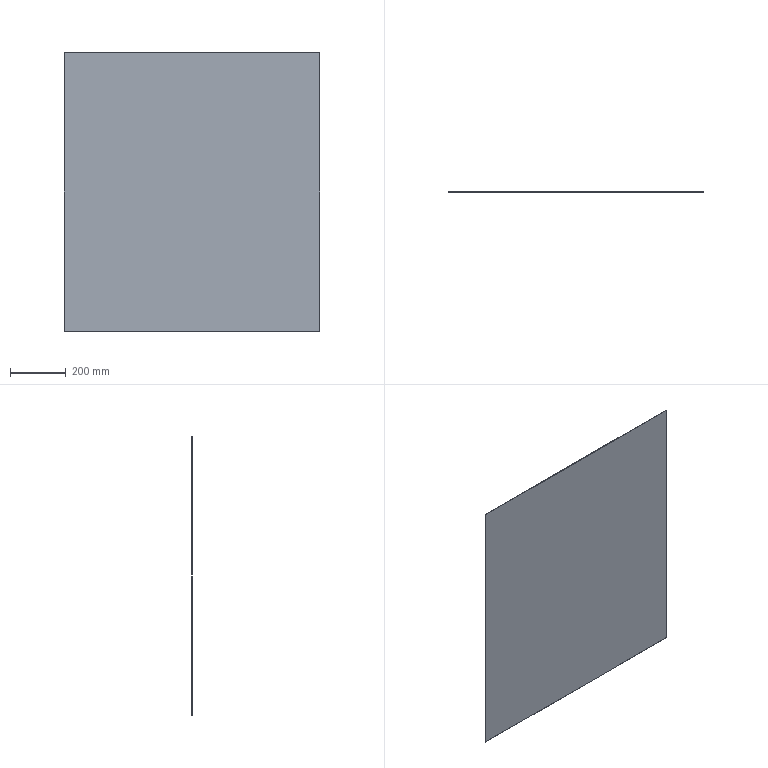Part | STEP file | 0243_Work-A | 1 solid | 6 faces | box 919 x 2.2 x 1000 mm | volume 2021800 mm3 | plane 6
STEP:
#1=CARTESIAN_POINT('',(0.,0.,0.));
#2=DIRECTION('',(0.,0.,1.));
#3=DIRECTION('',(1.,0.,0.));
#4=AXIS2_PLACEMENT_3D('',#1,#2,#3);
#5=CARTESIAN_POINT('',(0.,0.,-500.));
#6=VERTEX_POINT('',#5);
#7=CARTESIAN_POINT('',(0.,0.,500.));
#8=VERTEX_POINT('',#7);
#9=CARTESIAN_POINT('',(0.,0.,500.));
#10=DIRECTION('',(0.,0.,1.));
#11=VECTOR('',#10,1.);
#12=LINE('',#9,#11);
#13=CARTESIAN_POINT('',(0.,2.2,500.));
#14=DIRECTION('',(1.,0.,0.));
#15=DIRECTION('',(0.,0.,-1.));
#16=AXIS2_PLACEMENT_3D('',#13,#14,#15);
#17=PLANE('',#16);
#18=CARTESIAN_POINT('',(0.,-2.2));
#19=DIRECTION('',(-1.,0.));
#20=VECTOR('',#19,1.);
#21=LINE('',#18,#20);
#22=(GEOMETRIC_REPRESENTATION_CONTEXT(2)PARAMETRIC_REPRESENTATION_CONTEXT()REPRESENTATION_CONTEXT('',''));
#23=DEFINITIONAL_REPRESENTATION('',(#21),#22);
#24=PCURVE('',#17,#23);
#25=CARTESIAN_POINT('',(0.,0.,-500.));
#26=DIRECTION('',(0.,-1.,0.));
#27=DIRECTION('',(0.,0.,-1.));
#28=AXIS2_PLACEMENT_3D('',#25,#26,#27);
#29=PLANE('',#28);
#30=CARTESIAN_POINT('',(-1000.,0.));
#31=DIRECTION('',(-1.,0.));
#32=VECTOR('',#31,1.);
#33=LINE('',#30,#32);
#34=(GEOMETRIC_REPRESENTATION_CONTEXT(2)PARAMETRIC_REPRESENTATION_CONTEXT()REPRESENTATION_CONTEXT('',''));
#35=DEFINITIONAL_REPRESENTATION('',(#33),#34);
#36=PCURVE('',#29,#35);
#37=SURFACE_CURVE('',#12,(#24,#36),.PCURVE_S1.);
#38=EDGE_CURVE('',#6,#8,#37,.T.);
#39=ORIENTED_EDGE('',*,*,#38,.T.);
#40=CARTESIAN_POINT('',(0.,2.2,500.));
#41=VERTEX_POINT('',#40);
#42=CARTESIAN_POINT('',(0.,2.2,500.));
#43=DIRECTION('',(0.,-1.,0.));
#44=VECTOR('',#43,1.);
#45=LINE('',#42,#44);
#46=CARTESIAN_POINT('',(0.,0.));
#47=DIRECTION('',(0.,-1.));
#48=VECTOR('',#47,1.);
#49=LINE('',#46,#48);
#50=(GEOMETRIC_REPRESENTATION_CONTEXT(2)PARAMETRIC_REPRESENTATION_CONTEXT()REPRESENTATION_CONTEXT('',''));
#51=DEFINITIONAL_REPRESENTATION('',(#49),#50);
#52=PCURVE('',#17,#51);
#53=CARTESIAN_POINT('',(0.,2.2,500.));
#54=DIRECTION('',(0.,0.,-1.));
#55=DIRECTION('',(-1.,0.,0.));
#56=AXIS2_PLACEMENT_3D('',#53,#54,#55);
#57=PLANE('',#56);
#58=CARTESIAN_POINT('',(0.,0.));
#59=DIRECTION('',(0.,-1.));
#60=VECTOR('',#59,1.);
#61=LINE('',#58,#60);
#62=(GEOMETRIC_REPRESENTATION_CONTEXT(2)PARAMETRIC_REPRESENTATION_CONTEXT()REPRESENTATION_CONTEXT('',''));
#63=DEFINITIONAL_REPRESENTATION('',(#61),#62);
#64=PCURVE('',#57,#63);
#65=SURFACE_CURVE('',#45,(#52,#64),.PCURVE_S1.);
#66=EDGE_CURVE('',#41,#8,#65,.T.);
#67=ORIENTED_EDGE('',*,*,#66,.F.);
#68=CARTESIAN_POINT('',(0.,2.2,-500.));
#69=VERTEX_POINT('',#68);
#70=CARTESIAN_POINT('',(0.,2.2,500.));
#71=DIRECTION('',(0.,0.,1.));
#72=VECTOR('',#71,1.);
#73=LINE('',#70,#72);
#74=CARTESIAN_POINT('',(0.,0.));
#75=DIRECTION('',(-1.,0.));
#76=VECTOR('',#75,1.);
#77=LINE('',#74,#76);
#78=(GEOMETRIC_REPRESENTATION_CONTEXT(2)PARAMETRIC_REPRESENTATION_CONTEXT()REPRESENTATION_CONTEXT('',''));
#79=DEFINITIONAL_REPRESENTATION('',(#77),#78);
#80=PCURVE('',#17,#79);
#81=CARTESIAN_POINT('',(0.,2.2,-500.));
#82=DIRECTION('',(0.,-1.,0.));
#83=DIRECTION('',(0.,0.,-1.));
#84=AXIS2_PLACEMENT_3D('',#81,#82,#83);
#85=PLANE('',#84);
#86=CARTESIAN_POINT('',(-1000.,0.));
#87=DIRECTION('',(-1.,0.));
#88=VECTOR('',#87,1.);
#89=LINE('',#86,#88);
#90=(GEOMETRIC_REPRESENTATION_CONTEXT(2)PARAMETRIC_REPRESENTATION_CONTEXT()REPRESENTATION_CONTEXT('',''));
#91=DEFINITIONAL_REPRESENTATION('',(#89),#90);
#92=PCURVE('',#85,#91);
#93=SURFACE_CURVE('',#73,(#80,#92),.PCURVE_S1.);
#94=EDGE_CURVE('',#69,#41,#93,.T.);
#95=ORIENTED_EDGE('',*,*,#94,.F.);
#96=CARTESIAN_POINT('',(0.,2.2,-500.));
#97=DIRECTION('',(0.,-1.,0.));
#98=VECTOR('',#97,1.);
#99=LINE('',#96,#98);
#100=CARTESIAN_POINT('',(1000.,0.));
#101=DIRECTION('',(0.,-1.));
#102=VECTOR('',#101,1.);
#103=LINE('',#100,#102);
#104=(GEOMETRIC_REPRESENTATION_CONTEXT(2)PARAMETRIC_REPRESENTATION_CONTEXT()REPRESENTATION_CONTEXT('',''));
#105=DEFINITIONAL_REPRESENTATION('',(#103),#104);
#106=PCURVE('',#17,#105);
#107=CARTESIAN_POINT('',(0.,2.2,-500.));
#108=DIRECTION('',(0.,0.,1.));
#109=DIRECTION('',(1.,0.,0.));
#110=AXIS2_PLACEMENT_3D('',#107,#108,#109);
#111=PLANE('',#110);
#112=CARTESIAN_POINT('',(0.,0.));
#113=DIRECTION('',(0.,-1.));
#114=VECTOR('',#113,1.);
#115=LINE('',#112,#114);
#116=(GEOMETRIC_REPRESENTATION_CONTEXT(2)PARAMETRIC_REPRESENTATION_CONTEXT()REPRESENTATION_CONTEXT('',''));
#117=DEFINITIONAL_REPRESENTATION('',(#115),#116);
#118=PCURVE('',#111,#117);
#119=SURFACE_CURVE('',#99,(#106,#118),.PCURVE_S1.);
#120=EDGE_CURVE('',#69,#6,#119,.T.);
#121=ORIENTED_EDGE('',*,*,#120,.T.);
#122=EDGE_LOOP('',(#39,#67,#95,#121));
#123=FACE_BOUND('',#122,.T.);
#124=ADVANCED_FACE('',(#123),#17,.F.);
#125=CARTESIAN_POINT('',(919.,0.,500.));
#126=VERTEX_POINT('',#125);
#127=CARTESIAN_POINT('',(0.,0.,500.));
#128=DIRECTION('',(1.,0.,0.));
#129=VECTOR('',#128,1.);
#130=LINE('',#127,#129);
#131=CARTESIAN_POINT('',(0.,-2.2));
#132=DIRECTION('',(-1.,0.));
#133=VECTOR('',#132,1.);
#134=LINE('',#131,#133);
#135=(GEOMETRIC_REPRESENTATION_CONTEXT(2)PARAMETRIC_REPRESENTATION_CONTEXT()REPRESENTATION_CONTEXT('',''));
#136=DEFINITIONAL_REPRESENTATION('',(#134),#135);
#137=PCURVE('',#57,#136);
#138=CARTESIAN_POINT('',(-1000.,0.));
#139=DIRECTION('',(0.,1.));
#140=VECTOR('',#139,1.);
#141=LINE('',#138,#140);
#142=(GEOMETRIC_REPRESENTATION_CONTEXT(2)PARAMETRIC_REPRESENTATION_CONTEXT()REPRESENTATION_CONTEXT('',''));
#143=DEFINITIONAL_REPRESENTATION('',(#141),#142);
#144=PCURVE('',#29,#143);
#145=SURFACE_CURVE('',#130,(#137,#144),.PCURVE_S1.);
#146=EDGE_CURVE('',#8,#126,#145,.T.);
#147=ORIENTED_EDGE('',*,*,#146,.T.);
#148=CARTESIAN_POINT('',(919.,2.2,500.));
#149=VERTEX_POINT('',#148);
#150=CARTESIAN_POINT('',(919.,2.2,500.));
#151=DIRECTION('',(0.,-1.,0.));
#152=VECTOR('',#151,1.);
#153=LINE('',#150,#152);
#154=CARTESIAN_POINT('',(-919.,0.));
#155=DIRECTION('',(0.,-1.));
#156=VECTOR('',#155,1.);
#157=LINE('',#154,#156);
#158=(GEOMETRIC_REPRESENTATION_CONTEXT(2)PARAMETRIC_REPRESENTATION_CONTEXT()REPRESENTATION_CONTEXT('',''));
#159=DEFINITIONAL_REPRESENTATION('',(#157),#158);
#160=PCURVE('',#57,#159);
#161=CARTESIAN_POINT('',(919.,2.2,500.));
#162=DIRECTION('',(-1.,0.,0.));
#163=DIRECTION('',(0.,0.,1.));
#164=AXIS2_PLACEMENT_3D('',#161,#162,#163);
#165=PLANE('',#164);
#166=CARTESIAN_POINT('',(0.,0.));
#167=DIRECTION('',(0.,-1.));
#168=VECTOR('',#167,1.);
#169=LINE('',#166,#168);
#170=(GEOMETRIC_REPRESENTATION_CONTEXT(2)PARAMETRIC_REPRESENTATION_CONTEXT()REPRESENTATION_CONTEXT('',''));
#171=DEFINITIONAL_REPRESENTATION('',(#169),#170);
#172=PCURVE('',#165,#171);
#173=SURFACE_CURVE('',#153,(#160,#172),.PCURVE_S1.);
#174=EDGE_CURVE('',#149,#126,#173,.T.);
#175=ORIENTED_EDGE('',*,*,#174,.F.);
#176=CARTESIAN_POINT('',(0.,2.2,500.));
#177=DIRECTION('',(1.,0.,0.));
#178=VECTOR('',#177,1.);
#179=LINE('',#176,#178);
#180=CARTESIAN_POINT('',(0.,0.));
#181=DIRECTION('',(-1.,0.));
#182=VECTOR('',#181,1.);
#183=LINE('',#180,#182);
#184=(GEOMETRIC_REPRESENTATION_CONTEXT(2)PARAMETRIC_REPRESENTATION_CONTEXT()REPRESENTATION_CONTEXT('',''));
#185=DEFINITIONAL_REPRESENTATION('',(#183),#184);
#186=PCURVE('',#57,#185);
#187=CARTESIAN_POINT('',(-1000.,0.));
#188=DIRECTION('',(0.,1.));
#189=VECTOR('',#188,1.);
#190=LINE('',#187,#189);
#191=(GEOMETRIC_REPRESENTATION_CONTEXT(2)PARAMETRIC_REPRESENTATION_CONTEXT()REPRESENTATION_CONTEXT('',''));
#192=DEFINITIONAL_REPRESENTATION('',(#190),#191);
#193=PCURVE('',#85,#192);
#194=SURFACE_CURVE('',#179,(#186,#193),.PCURVE_S1.);
#195=EDGE_CURVE('',#41,#149,#194,.T.);
#196=ORIENTED_EDGE('',*,*,#195,.F.);
#197=ORIENTED_EDGE('',*,*,#66,.T.);
#198=EDGE_LOOP('',(#147,#175,#196,#197));
#199=FACE_BOUND('',#198,.T.);
#200=ADVANCED_FACE('',(#199),#57,.F.);
#201=CARTESIAN_POINT('',(919.,0.,-500.));
#202=VERTEX_POINT('',#201);
#203=CARTESIAN_POINT('',(919.,0.,500.));
#204=DIRECTION('',(0.,0.,-1.));
#205=VECTOR('',#204,1.);
#206=LINE('',#203,#205);
#207=CARTESIAN_POINT('',(0.,-2.2));
#208=DIRECTION('',(-1.,0.));
#209=VECTOR('',#208,1.);
#210=LINE('',#207,#209);
#211=(GEOMETRIC_REPRESENTATION_CONTEXT(2)PARAMETRIC_REPRESENTATION_CONTEXT()REPRESENTATION_CONTEXT('',''));
#212=DEFINITIONAL_REPRESENTATION('',(#210),#211);
#213=PCURVE('',#165,#212);
#214=CARTESIAN_POINT('',(-1000.,919.));
#215=DIRECTION('',(1.,0.));
#216=VECTOR('',#215,1.);
#217=LINE('',#214,#216);
#218=(GEOMETRIC_REPRESENTATION_CONTEXT(2)PARAMETRIC_REPRESENTATION_CONTEXT()REPRESENTATION_CONTEXT('',''));
#219=DEFINITIONAL_REPRESENTATION('',(#217),#218);
#220=PCURVE('',#29,#219);
#221=SURFACE_CURVE('',#206,(#213,#220),.PCURVE_S1.);
#222=EDGE_CURVE('',#126,#202,#221,.T.);
#223=ORIENTED_EDGE('',*,*,#222,.T.);
#224=CARTESIAN_POINT('',(919.,2.2,-500.));
#225=VERTEX_POINT('',#224);
#226=CARTESIAN_POINT('',(919.,2.2,-500.));
#227=DIRECTION('',(0.,-1.,0.));
#228=VECTOR('',#227,1.);
#229=LINE('',#226,#228);
#230=CARTESIAN_POINT('',(-1000.,0.));
#231=DIRECTION('',(0.,-1.));
#232=VECTOR('',#231,1.);
#233=LINE('',#230,#232);
#234=(GEOMETRIC_REPRESENTATION_CONTEXT(2)PARAMETRIC_REPRESENTATION_CONTEXT()REPRESENTATION_CONTEXT('',''));
#235=DEFINITIONAL_REPRESENTATION('',(#233),#234);
#236=PCURVE('',#165,#235);
#237=CARTESIAN_POINT('',(919.,0.));
#238=DIRECTION('',(0.,-1.));
#239=VECTOR('',#238,1.);
#240=LINE('',#237,#239);
#241=(GEOMETRIC_REPRESENTATION_CONTEXT(2)PARAMETRIC_REPRESENTATION_CONTEXT()REPRESENTATION_CONTEXT('',''));
#242=DEFINITIONAL_REPRESENTATION('',(#240),#241);
#243=PCURVE('',#111,#242);
#244=SURFACE_CURVE('',#229,(#236,#243),.PCURVE_S1.);
#245=EDGE_CURVE('',#225,#202,#244,.T.);
#246=ORIENTED_EDGE('',*,*,#245,.F.);
#247=CARTESIAN_POINT('',(919.,2.2,500.));
#248=DIRECTION('',(0.,0.,-1.));
#249=VECTOR('',#248,1.);
#250=LINE('',#247,#249);
#251=CARTESIAN_POINT('',(0.,0.));
#252=DIRECTION('',(-1.,0.));
#253=VECTOR('',#252,1.);
#254=LINE('',#251,#253);
#255=(GEOMETRIC_REPRESENTATION_CONTEXT(2)PARAMETRIC_REPRESENTATION_CONTEXT()REPRESENTATION_CONTEXT('',''));
#256=DEFINITIONAL_REPRESENTATION('',(#254),#255);
#257=PCURVE('',#165,#256);
#258=CARTESIAN_POINT('',(-1000.,919.));
#259=DIRECTION('',(1.,0.));
#260=VECTOR('',#259,1.);
#261=LINE('',#258,#260);
#262=(GEOMETRIC_REPRESENTATION_CONTEXT(2)PARAMETRIC_REPRESENTATION_CONTEXT()REPRESENTATION_CONTEXT('',''));
#263=DEFINITIONAL_REPRESENTATION('',(#261),#262);
#264=PCURVE('',#85,#263);
#265=SURFACE_CURVE('',#250,(#257,#264),.PCURVE_S1.);
#266=EDGE_CURVE('',#149,#225,#265,.T.);
#267=ORIENTED_EDGE('',*,*,#266,.F.);
#268=ORIENTED_EDGE('',*,*,#174,.T.);
#269=EDGE_LOOP('',(#223,#246,#267,#268));
#270=FACE_BOUND('',#269,.T.);
#271=ADVANCED_FACE('',(#270),#165,.F.);
#272=CARTESIAN_POINT('',(0.,0.,-500.));
#273=DIRECTION('',(-1.,0.,0.));
#274=VECTOR('',#273,1.);
#275=LINE('',#272,#274);
#276=CARTESIAN_POINT('',(0.,-2.2));
#277=DIRECTION('',(-1.,0.));
#278=VECTOR('',#277,1.);
#279=LINE('',#276,#278);
#280=(GEOMETRIC_REPRESENTATION_CONTEXT(2)PARAMETRIC_REPRESENTATION_CONTEXT()REPRESENTATION_CONTEXT('',''));
#281=DEFINITIONAL_REPRESENTATION('',(#279),#280);
#282=PCURVE('',#111,#281);
#283=CARTESIAN_POINT('',(0.,0.));
#284=DIRECTION('',(0.,-1.));
#285=VECTOR('',#284,1.);
#286=LINE('',#283,#285);
#287=(GEOMETRIC_REPRESENTATION_CONTEXT(2)PARAMETRIC_REPRESENTATION_CONTEXT()REPRESENTATION_CONTEXT('',''));
#288=DEFINITIONAL_REPRESENTATION('',(#286),#287);
#289=PCURVE('',#29,#288);
#290=SURFACE_CURVE('',#275,(#282,#289),.PCURVE_S1.);
#291=EDGE_CURVE('',#202,#6,#290,.T.);
#292=ORIENTED_EDGE('',*,*,#291,.T.);
#293=ORIENTED_EDGE('',*,*,#120,.F.);
#294=CARTESIAN_POINT('',(0.,2.2,-500.));
#295=DIRECTION('',(-1.,0.,0.));
#296=VECTOR('',#295,1.);
#297=LINE('',#294,#296);
#298=CARTESIAN_POINT('',(0.,0.));
#299=DIRECTION('',(-1.,0.));
#300=VECTOR('',#299,1.);
#301=LINE('',#298,#300);
#302=(GEOMETRIC_REPRESENTATION_CONTEXT(2)PARAMETRIC_REPRESENTATION_CONTEXT()REPRESENTATION_CONTEXT('',''));
#303=DEFINITIONAL_REPRESENTATION('',(#301),#302);
#304=PCURVE('',#111,#303);
#305=CARTESIAN_POINT('',(0.,0.));
#306=DIRECTION('',(0.,-1.));
#307=VECTOR('',#306,1.);
#308=LINE('',#305,#307);
#309=(GEOMETRIC_REPRESENTATION_CONTEXT(2)PARAMETRIC_REPRESENTATION_CONTEXT()REPRESENTATION_CONTEXT('',''));
#310=DEFINITIONAL_REPRESENTATION('',(#308),#309);
#311=PCURVE('',#85,#310);
#312=SURFACE_CURVE('',#297,(#304,#311),.PCURVE_S1.);
#313=EDGE_CURVE('',#225,#69,#312,.T.);
#314=ORIENTED_EDGE('',*,*,#313,.F.);
#315=ORIENTED_EDGE('',*,*,#245,.T.);
#316=EDGE_LOOP('',(#292,#293,#314,#315));
#317=FACE_BOUND('',#316,.T.);
#318=ADVANCED_FACE('',(#317),#111,.F.);
#319=ORIENTED_EDGE('',*,*,#94,.T.);
#320=ORIENTED_EDGE('',*,*,#195,.T.);
#321=ORIENTED_EDGE('',*,*,#266,.T.);
#322=ORIENTED_EDGE('',*,*,#313,.T.);
#323=EDGE_LOOP('',(#319,#320,#321,#322));
#324=FACE_BOUND('',#323,.T.);
#325=ADVANCED_FACE('',(#324),#85,.F.);
#326=ORIENTED_EDGE('',*,*,#38,.F.);
#327=ORIENTED_EDGE('',*,*,#291,.F.);
#328=ORIENTED_EDGE('',*,*,#222,.F.);
#329=ORIENTED_EDGE('',*,*,#146,.F.);
#330=EDGE_LOOP('',(#326,#327,#328,#329));
#331=FACE_BOUND('',#330,.T.);
#332=ADVANCED_FACE('',(#331),#29,.T.);
#333=CLOSED_SHELL('',(#124,#200,#271,#318,#325,#332));
#334=MANIFOLD_SOLID_BREP('',#333);
#335=(LENGTH_UNIT()NAMED_UNIT(*)SI_UNIT(.MILLI.,.METRE.));
#336=UNCERTAINTY_MEASURE_WITH_UNIT(LENGTH_MEASURE(0.0000001),#335,'','');
#337=(NAMED_UNIT(*)PLANE_ANGLE_UNIT()SI_UNIT($,.RADIAN.));
#338=(NAMED_UNIT(*)SI_UNIT($,.STERADIAN.)SOLID_ANGLE_UNIT());
#339=(GEOMETRIC_REPRESENTATION_CONTEXT(3)GLOBAL_UNCERTAINTY_ASSIGNED_CONTEXT((#336))GLOBAL_UNIT_ASSIGNED_CONTEXT((#335,#337,#338))REPRESENTATION_CONTEXT('',''));
#340=ADVANCED_BREP_SHAPE_REPRESENTATION('',(#4,#334),#339);